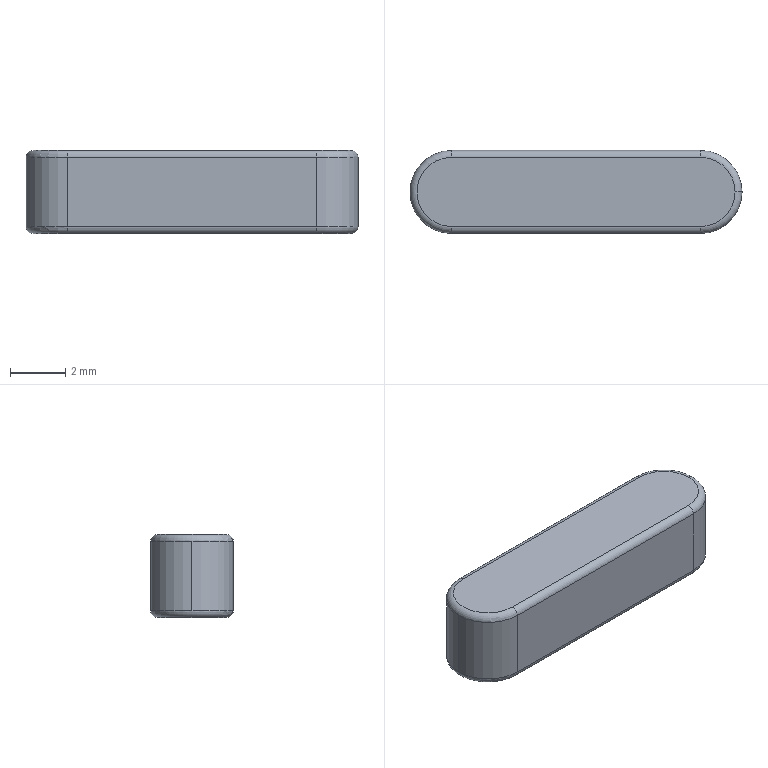Part | STEP file | Type A plain parallel key GB/T 1096 - key 3x3x12 | 1 solid | 17 faces | box 12 x 3 x 3 mm | volume 101.479 mm3 | cylinder 7 | torus 6 | plane 4 | commonest cylinder face diameters 0.5 x4 3 x3
STEP:
#1=CARTESIAN_POINT('',(0.,0.,0.));
#2=DIRECTION('',(0.,0.,1.));
#3=DIRECTION('',(1.,0.,0.));
#4=AXIS2_PLACEMENT_3D('',#1,#2,#3);
#5=CARTESIAN_POINT('',(5.75,0.,0.));
#6=VERTEX_POINT('',#5);
#7=CARTESIAN_POINT('',(4.5,-1.25,0.));
#8=VERTEX_POINT('',#7);
#9=CARTESIAN_POINT('',(4.5,0.,0.));
#10=DIRECTION('',(0.,0.,-1.));
#11=DIRECTION('',(1.,0.,0.));
#12=AXIS2_PLACEMENT_3D('',#9,#10,#11);
#13=CIRCLE('',#12,1.25);
#14=CARTESIAN_POINT('',(4.5,0.,0.25));
#15=DIRECTION('',(0.,0.,1.));
#16=DIRECTION('',(1.,0.,0.));
#17=AXIS2_PLACEMENT_3D('',#14,#15,#16);
#18=TOROIDAL_SURFACE('',#17,1.25,0.25);
#19=CARTESIAN_POINT('',(6.283,4.712));
#20=DIRECTION('',(-1.,0.));
#21=VECTOR('',#20,1.);
#22=LINE('',#19,#21);
#23=(GEOMETRIC_REPRESENTATION_CONTEXT(2)PARAMETRIC_REPRESENTATION_CONTEXT()REPRESENTATION_CONTEXT('',''));
#24=DEFINITIONAL_REPRESENTATION('',(#22),#23);
#25=PCURVE('',#18,#24);
#26=CARTESIAN_POINT('',(-4.5,0.,0.));
#27=DIRECTION('',(0.,0.,1.));
#28=DIRECTION('',(1.,0.,0.));
#29=AXIS2_PLACEMENT_3D('',#26,#27,#28);
#30=PLANE('',#29);
#31=CARTESIAN_POINT('',(10.25,0.));
#32=CARTESIAN_POINT('',(10.25,-2.165));
#33=CARTESIAN_POINT('',(8.375,-1.083));
#34=CARTESIAN_POINT('',(6.5,0.));
#35=CARTESIAN_POINT('',(8.375,1.083));
#36=CARTESIAN_POINT('',(10.25,2.165));
#37=CARTESIAN_POINT('',(10.25,0.));
#38=(BOUNDED_CURVE()B_SPLINE_CURVE(2,(#31,#32,#33,#34,#35,#36,#37),.UNSPECIFIED.,.T.,.F.)B_SPLINE_CURVE_WITH_KNOTS((1,2,2,2,2,1),(-2.094,0.,2.094,4.189,6.283,8.378),.UNSPECIFIED.)CURVE()GEOMETRIC_REPRESENTATION_ITEM()RATIONAL_B_SPLINE_CURVE((1.,0.5,1.,0.5,1.,0.5,1.))REPRESENTATION_ITEM(''));
#39=(GEOMETRIC_REPRESENTATION_CONTEXT(2)PARAMETRIC_REPRESENTATION_CONTEXT()REPRESENTATION_CONTEXT('',''));
#40=DEFINITIONAL_REPRESENTATION('',(#38),#39);
#41=PCURVE('',#30,#40);
#42=SURFACE_CURVE('',#13,(#25,#41),.PCURVE_S1.);
#43=EDGE_CURVE('',#6,#8,#42,.T.);
#44=ORIENTED_EDGE('',*,*,#43,.F.);
#45=CARTESIAN_POINT('',(6.,0.,0.25));
#46=VERTEX_POINT('',#45);
#47=CARTESIAN_POINT('',(5.75,0.,0.25));
#48=DIRECTION('',(0.,-1.,0.));
#49=DIRECTION('',(0.,0.,-1.));
#50=AXIS2_PLACEMENT_3D('',#47,#48,#49);
#51=CIRCLE('',#50,0.25);
#52=CARTESIAN_POINT('',(6.283,4.712));
#53=DIRECTION('',(0.,1.));
#54=VECTOR('',#53,1.);
#55=LINE('',#52,#54);
#56=(GEOMETRIC_REPRESENTATION_CONTEXT(2)PARAMETRIC_REPRESENTATION_CONTEXT()REPRESENTATION_CONTEXT('',''));
#57=DEFINITIONAL_REPRESENTATION('',(#55),#56);
#58=PCURVE('',#18,#57);
#59=CARTESIAN_POINT('',(4.5,0.,0.25));
#60=DIRECTION('',(0.,0.,1.));
#61=DIRECTION('',(1.,0.,0.));
#62=AXIS2_PLACEMENT_3D('',#59,#60,#61);
#63=TOROIDAL_SURFACE('',#62,1.25,0.25);
#64=CARTESIAN_POINT('',(0.,4.712));
#65=DIRECTION('',(0.,1.));
#66=VECTOR('',#65,1.);
#67=LINE('',#64,#66);
#68=(GEOMETRIC_REPRESENTATION_CONTEXT(2)PARAMETRIC_REPRESENTATION_CONTEXT()REPRESENTATION_CONTEXT('',''));
#69=DEFINITIONAL_REPRESENTATION('',(#67),#68);
#70=PCURVE('',#63,#69);
#71=SURFACE_CURVE('',#51,(#58,#70),.PCURVE_S1.);
#72=EDGE_CURVE('',#6,#46,#71,.T.);
#73=ORIENTED_EDGE('',*,*,#72,.T.);
#74=CARTESIAN_POINT('',(4.5,-1.5,0.25));
#75=VERTEX_POINT('',#74);
#76=CARTESIAN_POINT('',(4.5,0.,0.25));
#77=DIRECTION('',(0.,0.,1.));
#78=DIRECTION('',(1.,0.,0.));
#79=AXIS2_PLACEMENT_3D('',#76,#77,#78);
#80=CIRCLE('',#79,1.5);
#81=CARTESIAN_POINT('',(0.,6.283));
#82=DIRECTION('',(1.,0.));
#83=VECTOR('',#82,1.);
#84=LINE('',#81,#83);
#85=(GEOMETRIC_REPRESENTATION_CONTEXT(2)PARAMETRIC_REPRESENTATION_CONTEXT()REPRESENTATION_CONTEXT('',''));
#86=DEFINITIONAL_REPRESENTATION('',(#84),#85);
#87=PCURVE('',#18,#86);
#88=CARTESIAN_POINT('',(4.5,0.,3.));
#89=DIRECTION('',(0.,0.,-1.));
#90=DIRECTION('',(-1.,0.,0.));
#91=AXIS2_PLACEMENT_3D('',#88,#89,#90);
#92=CYLINDRICAL_SURFACE('',#91,1.5);
#93=CARTESIAN_POINT('',(9.425,2.75));
#94=DIRECTION('',(-1.,0.));
#95=VECTOR('',#94,1.);
#96=LINE('',#93,#95);
#97=(GEOMETRIC_REPRESENTATION_CONTEXT(2)PARAMETRIC_REPRESENTATION_CONTEXT()REPRESENTATION_CONTEXT('',''));
#98=DEFINITIONAL_REPRESENTATION('',(#96),#97);
#99=PCURVE('',#92,#98);
#100=SURFACE_CURVE('',#80,(#87,#99),.PCURVE_S1.);
#101=EDGE_CURVE('',#75,#46,#100,.T.);
#102=ORIENTED_EDGE('',*,*,#101,.F.);
#103=CARTESIAN_POINT('',(4.5,-1.25,0.25));
#104=DIRECTION('',(1.,0.,0.));
#105=DIRECTION('',(0.,0.,-1.));
#106=AXIS2_PLACEMENT_3D('',#103,#104,#105);
#107=CIRCLE('',#106,0.25);
#108=CARTESIAN_POINT('',(4.712,10.996));
#109=DIRECTION('',(0.,-1.));
#110=VECTOR('',#109,1.);
#111=LINE('',#108,#110);
#112=(GEOMETRIC_REPRESENTATION_CONTEXT(2)PARAMETRIC_REPRESENTATION_CONTEXT()REPRESENTATION_CONTEXT('',''));
#113=DEFINITIONAL_REPRESENTATION('',(#111),#112);
#114=PCURVE('',#18,#113);
#115=CARTESIAN_POINT('',(-4.5,-1.25,0.25));
#116=DIRECTION('',(1.,0.,0.));
#117=DIRECTION('',(0.,1.,0.));
#118=AXIS2_PLACEMENT_3D('',#115,#116,#117);
#119=CYLINDRICAL_SURFACE('',#118,0.25);
#120=CARTESIAN_POINT('',(-1.571,9.));
#121=DIRECTION('',(1.,0.));
#122=VECTOR('',#121,1.);
#123=LINE('',#120,#122);
#124=(GEOMETRIC_REPRESENTATION_CONTEXT(2)PARAMETRIC_REPRESENTATION_CONTEXT()REPRESENTATION_CONTEXT('',''));
#125=DEFINITIONAL_REPRESENTATION('',(#123),#124);
#126=PCURVE('',#119,#125);
#127=SURFACE_CURVE('',#107,(#114,#126),.PCURVE_S1.);
#128=EDGE_CURVE('',#75,#8,#127,.T.);
#129=ORIENTED_EDGE('',*,*,#128,.T.);
#130=EDGE_LOOP('',(#44,#73,#102,#129));
#131=FACE_BOUND('',#130,.T.);
#132=ADVANCED_FACE('',(#131),#18,.T.);
#133=CARTESIAN_POINT('',(6.,0.,2.75));
#134=VERTEX_POINT('',#133);
#135=CARTESIAN_POINT('',(4.5,-1.5,2.75));
#136=VERTEX_POINT('',#135);
#137=CARTESIAN_POINT('',(4.5,0.,2.75));
#138=DIRECTION('',(0.,0.,-1.));
#139=DIRECTION('',(1.,0.,0.));
#140=AXIS2_PLACEMENT_3D('',#137,#138,#139);
#141=CIRCLE('',#140,1.5);
#142=CARTESIAN_POINT('',(4.5,0.,2.75));
#143=DIRECTION('',(0.,0.,1.));
#144=DIRECTION('',(1.,0.,0.));
#145=AXIS2_PLACEMENT_3D('',#142,#143,#144);
#146=TOROIDAL_SURFACE('',#145,1.25,0.25);
#147=CARTESIAN_POINT('',(6.283,0.));
#148=DIRECTION('',(-1.,0.));
#149=VECTOR('',#148,1.);
#150=LINE('',#147,#149);
#151=(GEOMETRIC_REPRESENTATION_CONTEXT(2)PARAMETRIC_REPRESENTATION_CONTEXT()REPRESENTATION_CONTEXT('',''));
#152=DEFINITIONAL_REPRESENTATION('',(#150),#151);
#153=PCURVE('',#146,#152);
#154=CARTESIAN_POINT('',(3.142,0.25));
#155=DIRECTION('',(1.,0.));
#156=VECTOR('',#155,1.);
#157=LINE('',#154,#156);
#158=(GEOMETRIC_REPRESENTATION_CONTEXT(2)PARAMETRIC_REPRESENTATION_CONTEXT()REPRESENTATION_CONTEXT('',''));
#159=DEFINITIONAL_REPRESENTATION('',(#157),#158);
#160=PCURVE('',#92,#159);
#161=SURFACE_CURVE('',#141,(#153,#160),.PCURVE_S1.);
#162=EDGE_CURVE('',#134,#136,#161,.T.);
#163=ORIENTED_EDGE('',*,*,#162,.F.);
#164=CARTESIAN_POINT('',(5.75,0.,3.));
#165=VERTEX_POINT('',#164);
#166=CARTESIAN_POINT('',(5.75,0.,2.75));
#167=DIRECTION('',(0.,-1.,0.));
#168=DIRECTION('',(0.,0.,-1.));
#169=AXIS2_PLACEMENT_3D('',#166,#167,#168);
#170=CIRCLE('',#169,0.25);
#171=CARTESIAN_POINT('',(6.283,-1.571));
#172=DIRECTION('',(0.,1.));
#173=VECTOR('',#172,1.);
#174=LINE('',#171,#173);
#175=(GEOMETRIC_REPRESENTATION_CONTEXT(2)PARAMETRIC_REPRESENTATION_CONTEXT()REPRESENTATION_CONTEXT('',''));
#176=DEFINITIONAL_REPRESENTATION('',(#174),#175);
#177=PCURVE('',#146,#176);
#178=CARTESIAN_POINT('',(4.5,0.,2.75));
#179=DIRECTION('',(0.,0.,1.));
#180=DIRECTION('',(1.,0.,0.));
#181=AXIS2_PLACEMENT_3D('',#178,#179,#180);
#182=TOROIDAL_SURFACE('',#181,1.25,0.25);
#183=CARTESIAN_POINT('',(0.,-1.571));
#184=DIRECTION('',(0.,1.));
#185=VECTOR('',#184,1.);
#186=LINE('',#183,#185);
#187=(GEOMETRIC_REPRESENTATION_CONTEXT(2)PARAMETRIC_REPRESENTATION_CONTEXT()REPRESENTATION_CONTEXT('',''));
#188=DEFINITIONAL_REPRESENTATION('',(#186),#187);
#189=PCURVE('',#182,#188);
#190=SURFACE_CURVE('',#170,(#177,#189),.PCURVE_S1.);
#191=EDGE_CURVE('',#134,#165,#190,.T.);
#192=ORIENTED_EDGE('',*,*,#191,.T.);
#193=CARTESIAN_POINT('',(4.5,-1.25,3.));
#194=VERTEX_POINT('',#193);
#195=CARTESIAN_POINT('',(4.5,0.,3.));
#196=DIRECTION('',(0.,0.,1.));
#197=DIRECTION('',(1.,0.,0.));
#198=AXIS2_PLACEMENT_3D('',#195,#196,#197);
#199=CIRCLE('',#198,1.25);
#200=CARTESIAN_POINT('',(0.,1.571));
#201=DIRECTION('',(1.,0.));
#202=VECTOR('',#201,1.);
#203=LINE('',#200,#202);
#204=(GEOMETRIC_REPRESENTATION_CONTEXT(2)PARAMETRIC_REPRESENTATION_CONTEXT()REPRESENTATION_CONTEXT('',''));
#205=DEFINITIONAL_REPRESENTATION('',(#203),#204);
#206=PCURVE('',#146,#205);
#207=CARTESIAN_POINT('',(-4.5,0.,3.));
#208=DIRECTION('',(0.,0.,1.));
#209=DIRECTION('',(1.,0.,0.));
#210=AXIS2_PLACEMENT_3D('',#207,#208,#209);
#211=PLANE('',#210);
#212=CARTESIAN_POINT('',(9.,0.));
#213=DIRECTION('',(1.,0.));
#214=AXIS2_PLACEMENT_2D('',#212,#213);
#215=CIRCLE('',#214,1.25);
#216=(GEOMETRIC_REPRESENTATION_CONTEXT(2)PARAMETRIC_REPRESENTATION_CONTEXT()REPRESENTATION_CONTEXT('',''));
#217=DEFINITIONAL_REPRESENTATION('',(#215),#216);
#218=PCURVE('',#211,#217);
#219=SURFACE_CURVE('',#199,(#206,#218),.PCURVE_S1.);
#220=EDGE_CURVE('',#194,#165,#219,.T.);
#221=ORIENTED_EDGE('',*,*,#220,.F.);
#222=CARTESIAN_POINT('',(4.5,-1.25,2.75));
#223=DIRECTION('',(1.,0.,0.));
#224=DIRECTION('',(0.,0.,-1.));
#225=AXIS2_PLACEMENT_3D('',#222,#223,#224);
#226=CIRCLE('',#225,0.25);
#227=CARTESIAN_POINT('',(4.712,4.712));
#228=DIRECTION('',(0.,-1.));
#229=VECTOR('',#228,1.);
#230=LINE('',#227,#229);
#231=(GEOMETRIC_REPRESENTATION_CONTEXT(2)PARAMETRIC_REPRESENTATION_CONTEXT()REPRESENTATION_CONTEXT('',''));
#232=DEFINITIONAL_REPRESENTATION('',(#230),#231);
#233=PCURVE('',#146,#232);
#234=CARTESIAN_POINT('',(-4.5,-1.25,2.75));
#235=DIRECTION('',(-1.,0.,0.));
#236=DIRECTION('',(0.,-1.,0.));
#237=AXIS2_PLACEMENT_3D('',#234,#235,#236);
#238=CYLINDRICAL_SURFACE('',#237,0.25);
#239=CARTESIAN_POINT('',(4.712,-9.));
#240=DIRECTION('',(-1.,0.));
#241=VECTOR('',#240,1.);
#242=LINE('',#239,#241);
#243=(GEOMETRIC_REPRESENTATION_CONTEXT(2)PARAMETRIC_REPRESENTATION_CONTEXT()REPRESENTATION_CONTEXT('',''));
#244=DEFINITIONAL_REPRESENTATION('',(#242),#243);
#245=PCURVE('',#238,#244);
#246=SURFACE_CURVE('',#226,(#233,#245),.PCURVE_S1.);
#247=EDGE_CURVE('',#194,#136,#246,.T.);
#248=ORIENTED_EDGE('',*,*,#247,.T.);
#249=EDGE_LOOP('',(#163,#192,#221,#248));
#250=FACE_BOUND('',#249,.T.);
#251=ADVANCED_FACE('',(#250),#146,.T.);
#252=CARTESIAN_POINT('',(-4.5,-1.5,2.75));
#253=VERTEX_POINT('',#252);
#254=CARTESIAN_POINT('',(-6.,0.,2.75));
#255=VERTEX_POINT('',#254);
#256=CARTESIAN_POINT('',(-4.5,0.,2.75));
#257=DIRECTION('',(0.,0.,-1.));
#258=DIRECTION('',(1.,0.,0.));
#259=AXIS2_PLACEMENT_3D('',#256,#257,#258);
#260=CIRCLE('',#259,1.5);
#261=CARTESIAN_POINT('',(-4.5,0.,3.));
#262=DIRECTION('',(0.,0.,-1.));
#263=DIRECTION('',(-1.,0.,0.));
#264=AXIS2_PLACEMENT_3D('',#261,#262,#263);
#265=CYLINDRICAL_SURFACE('',#264,1.5);
#266=CARTESIAN_POINT('',(3.142,0.25));
#267=DIRECTION('',(1.,0.));
#268=VECTOR('',#267,1.);
#269=LINE('',#266,#268);
#270=(GEOMETRIC_REPRESENTATION_CONTEXT(2)PARAMETRIC_REPRESENTATION_CONTEXT()REPRESENTATION_CONTEXT('',''));
#271=DEFINITIONAL_REPRESENTATION('',(#269),#270);
#272=PCURVE('',#265,#271);
#273=CARTESIAN_POINT('',(-4.5,0.,2.75));
#274=DIRECTION('',(0.,0.,1.));
#275=DIRECTION('',(1.,0.,0.));
#276=AXIS2_PLACEMENT_3D('',#273,#274,#275);
#277=TOROIDAL_SURFACE('',#276,1.25,0.25);
#278=CARTESIAN_POINT('',(6.283,0.));
#279=DIRECTION('',(-1.,0.));
#280=VECTOR('',#279,1.);
#281=LINE('',#278,#280);
#282=(GEOMETRIC_REPRESENTATION_CONTEXT(2)PARAMETRIC_REPRESENTATION_CONTEXT()REPRESENTATION_CONTEXT('',''));
#283=DEFINITIONAL_REPRESENTATION('',(#281),#282);
#284=PCURVE('',#277,#283);
#285=SURFACE_CURVE('',#260,(#272,#284),.PCURVE_S1.);
#286=EDGE_CURVE('',#253,#255,#285,.T.);
#287=ORIENTED_EDGE('',*,*,#286,.T.);
#288=CARTESIAN_POINT('',(-6.,0.,0.25));
#289=VERTEX_POINT('',#288);
#290=CARTESIAN_POINT('',(-6.,0.,3.));
#291=DIRECTION('',(0.,0.,-1.));
#292=VECTOR('',#291,1.);
#293=LINE('',#290,#292);
#294=CARTESIAN_POINT('',(6.283,0.));
#295=DIRECTION('',(0.,1.));
#296=VECTOR('',#295,1.);
#297=LINE('',#294,#296);
#298=(GEOMETRIC_REPRESENTATION_CONTEXT(2)PARAMETRIC_REPRESENTATION_CONTEXT()REPRESENTATION_CONTEXT('',''));
#299=DEFINITIONAL_REPRESENTATION('',(#297),#298);
#300=PCURVE('',#265,#299);
#301=CARTESIAN_POINT('',(-4.5,0.,3.));
#302=DIRECTION('',(0.,0.,-1.));
#303=DIRECTION('',(-1.,0.,0.));
#304=AXIS2_PLACEMENT_3D('',#301,#302,#303);
#305=CYLINDRICAL_SURFACE('',#304,1.5);
#306=CARTESIAN_POINT('',(0.,0.));
#307=DIRECTION('',(0.,1.));
#308=VECTOR('',#307,1.);
#309=LINE('',#306,#308);
#310=(GEOMETRIC_REPRESENTATION_CONTEXT(2)PARAMETRIC_REPRESENTATION_CONTEXT()REPRESENTATION_CONTEXT('',''));
#311=DEFINITIONAL_REPRESENTATION('',(#309),#310);
#312=PCURVE('',#305,#311);
#313=SURFACE_CURVE('',#293,(#300,#312),.PCURVE_S1.);
#314=EDGE_CURVE('',#255,#289,#313,.T.);
#315=ORIENTED_EDGE('',*,*,#314,.T.);
#316=CARTESIAN_POINT('',(-4.5,-1.5,0.25));
#317=VERTEX_POINT('',#316);
#318=CARTESIAN_POINT('',(-4.5,0.,0.25));
#319=DIRECTION('',(0.,0.,1.));
#320=DIRECTION('',(1.,0.,0.));
#321=AXIS2_PLACEMENT_3D('',#318,#319,#320);
#322=CIRCLE('',#321,1.5);
#323=CARTESIAN_POINT('',(9.425,2.75));
#324=DIRECTION('',(-1.,0.));
#325=VECTOR('',#324,1.);
#326=LINE('',#323,#325);
#327=(GEOMETRIC_REPRESENTATION_CONTEXT(2)PARAMETRIC_REPRESENTATION_CONTEXT()REPRESENTATION_CONTEXT('',''));
#328=DEFINITIONAL_REPRESENTATION('',(#326),#327);
#329=PCURVE('',#265,#328);
#330=CARTESIAN_POINT('',(-4.5,0.,0.25));
#331=DIRECTION('',(0.,0.,1.));
#332=DIRECTION('',(1.,0.,0.));
#333=AXIS2_PLACEMENT_3D('',#330,#331,#332);
#334=TOROIDAL_SURFACE('',#333,1.25,0.25);
#335=CARTESIAN_POINT('',(0.,6.283));
#336=DIRECTION('',(1.,0.));
#337=VECTOR('',#336,1.);
#338=LINE('',#335,#337);
#339=(GEOMETRIC_REPRESENTATION_CONTEXT(2)PARAMETRIC_REPRESENTATION_CONTEXT()REPRESENTATION_CONTEXT('',''));
#340=DEFINITIONAL_REPRESENTATION('',(#338),#339);
#341=PCURVE('',#334,#340);
#342=SURFACE_CURVE('',#322,(#329,#341),.PCURVE_S1.);
#343=EDGE_CURVE('',#289,#317,#342,.T.);
#344=ORIENTED_EDGE('',*,*,#343,.T.);
#345=CARTESIAN_POINT('',(-4.5,-1.5,3.));
#346=DIRECTION('',(0.,0.,-1.));
#347=VECTOR('',#346,1.);
#348=LINE('',#345,#347);
#349=CARTESIAN_POINT('',(4.712,0.));
#350=DIRECTION('',(0.,1.));
#351=VECTOR('',#350,1.);
#352=LINE('',#349,#351);
#353=(GEOMETRIC_REPRESENTATION_CONTEXT(2)PARAMETRIC_REPRESENTATION_CONTEXT()REPRESENTATION_CONTEXT('',''));
#354=DEFINITIONAL_REPRESENTATION('',(#352),#353);
#355=PCURVE('',#265,#354);
#356=CARTESIAN_POINT('',(-4.5,-1.5,3.));
#357=DIRECTION('',(0.,1.,0.));
#358=DIRECTION('',(-1.,0.,0.));
#359=AXIS2_PLACEMENT_3D('',#356,#357,#358);
#360=PLANE('',#359);
#361=CARTESIAN_POINT('',(0.,0.));
#362=DIRECTION('',(0.,-1.));
#363=VECTOR('',#362,1.);
#364=LINE('',#361,#363);
#365=(GEOMETRIC_REPRESENTATION_CONTEXT(2)PARAMETRIC_REPRESENTATION_CONTEXT()REPRESENTATION_CONTEXT('',''));
#366=DEFINITIONAL_REPRESENTATION('',(#364),#365);
#367=PCURVE('',#360,#366);
#368=SURFACE_CURVE('',#348,(#355,#367),.PCURVE_S1.);
#369=EDGE_CURVE('',#253,#317,#368,.T.);
#370=ORIENTED_EDGE('',*,*,#369,.F.);
#371=EDGE_LOOP('',(#287,#315,#344,#370));
#372=FACE_BOUND('',#371,.T.);
#373=ADVANCED_FACE('',(#372),#265,.T.);
#374=ORIENTED_EDGE('',*,*,#314,.F.);
#375=CARTESIAN_POINT('',(-4.5,1.5,2.75));
#376=VERTEX_POINT('',#375);
#377=CARTESIAN_POINT('',(-4.5,0.,2.75));
#378=DIRECTION('',(0.,0.,-1.));
#379=DIRECTION('',(1.,0.,0.));
#380=AXIS2_PLACEMENT_3D('',#377,#378,#379);
#381=CIRCLE('',#380,1.5);
#382=CARTESIAN_POINT('',(-3.142,0.25));
#383=DIRECTION('',(1.,0.));
#384=VECTOR('',#383,1.);
#385=LINE('',#382,#384);
#386=(GEOMETRIC_REPRESENTATION_CONTEXT(2)PARAMETRIC_REPRESENTATION_CONTEXT()REPRESENTATION_CONTEXT('',''));
#387=DEFINITIONAL_REPRESENTATION('',(#385),#386);
#388=PCURVE('',#305,#387);
#389=CARTESIAN_POINT('',(6.283,0.));
#390=DIRECTION('',(-1.,0.));
#391=VECTOR('',#390,1.);
#392=LINE('',#389,#391);
#393=(GEOMETRIC_REPRESENTATION_CONTEXT(2)PARAMETRIC_REPRESENTATION_CONTEXT()REPRESENTATION_CONTEXT('',''));
#394=DEFINITIONAL_REPRESENTATION('',(#392),#393);
#395=PCURVE('',#277,#394);
#396=SURFACE_CURVE('',#381,(#388,#395),.PCURVE_S1.);
#397=EDGE_CURVE('',#255,#376,#396,.T.);
#398=ORIENTED_EDGE('',*,*,#397,.T.);
#399=CARTESIAN_POINT('',(-4.5,1.5,0.25));
#400=VERTEX_POINT('',#399);
#401=CARTESIAN_POINT('',(-4.5,1.5,3.));
#402=DIRECTION('',(0.,0.,-1.));
#403=VECTOR('',#402,1.);
#404=LINE('',#401,#403);
#405=CARTESIAN_POINT('',(1.571,0.));
#406=DIRECTION('',(0.,1.));
#407=VECTOR('',#406,1.);
#408=LINE('',#405,#407);
#409=(GEOMETRIC_REPRESENTATION_CONTEXT(2)PARAMETRIC_REPRESENTATION_CONTEXT()REPRESENTATION_CONTEXT('',''));
#410=DEFINITIONAL_REPRESENTATION('',(#408),#409);
#411=PCURVE('',#305,#410);
#412=CARTESIAN_POINT('',(-4.5,1.5,3.));
#413=DIRECTION('',(0.,-1.,0.));
#414=DIRECTION('',(1.,0.,0.));
#415=AXIS2_PLACEMENT_3D('',#412,#413,#414);
#416=PLANE('',#415);
#417=CARTESIAN_POINT('',(0.,0.));
#418=DIRECTION('',(0.,-1.));
#419=VECTOR('',#418,1.);
#420=LINE('',#417,#419);
#421=(GEOMETRIC_REPRESENTATION_CONTEXT(2)PARAMETRIC_REPRESENTATION_CONTEXT()REPRESENTATION_CONTEXT('',''));
#422=DEFINITIONAL_REPRESENTATION('',(#420),#421);
#423=PCURVE('',#416,#422);
#424=SURFACE_CURVE('',#404,(#411,#423),.PCURVE_S1.);
#425=EDGE_CURVE('',#376,#400,#424,.T.);
#426=ORIENTED_EDGE('',*,*,#425,.T.);
#427=CARTESIAN_POINT('',(-4.5,0.,0.25));
#428=DIRECTION('',(0.,0.,1.));
#429=DIRECTION('',(1.,0.,0.));
#430=AXIS2_PLACEMENT_3D('',#427,#428,#429);
#431=CIRCLE('',#430,1.5);
#432=CARTESIAN_POINT('',(3.142,2.75));
#433=DIRECTION('',(-1.,0.));
#434=VECTOR('',#433,1.);
#435=LINE('',#432,#434);
#436=(GEOMETRIC_REPRESENTATION_CONTEXT(2)PARAMETRIC_REPRESENTATION_CONTEXT()REPRESENTATION_CONTEXT('',''));
#437=DEFINITIONAL_REPRESENTATION('',(#435),#436);
#438=PCURVE('',#305,#437);
#439=CARTESIAN_POINT('',(0.,6.283));
#440=DIRECTION('',(1.,0.));
#441=VECTOR('',#440,1.);
#442=LINE('',#439,#441);
#443=(GEOMETRIC_REPRESENTATION_CONTEXT(2)PARAMETRIC_REPRESENTATION_CONTEXT()REPRESENTATION_CONTEXT('',''));
#444=DEFINITIONAL_REPRESENTATION('',(#442),#443);
#445=PCURVE('',#334,#444);
#446=SURFACE_CURVE('',#431,(#438,#445),.PCURVE_S1.);
#447=EDGE_CURVE('',#400,#289,#446,.T.);
#448=ORIENTED_EDGE('',*,*,#447,.T.);
#449=EDGE_LOOP('',(#374,#398,#426,#448));
#450=FACE_BOUND('',#449,.T.);
#451=ADVANCED_FACE('',(#450),#305,.T.);
#452=CARTESIAN_POINT('',(4.5,-1.5,3.));
#453=DIRECTION('',(0.,0.,-1.));
#454=VECTOR('',#453,1.);
#455=LINE('',#452,#454);
#456=CARTESIAN_POINT('',(-9.,0.));
#457=DIRECTION('',(0.,-1.));
#458=VECTOR('',#457,1.);
#459=LINE('',#456,#458);
#460=(GEOMETRIC_REPRESENTATION_CONTEXT(2)PARAMETRIC_REPRESENTATION_CONTEXT()REPRESENTATION_CONTEXT('',''));
#461=DEFINITIONAL_REPRESENTATION('',(#459),#460);
#462=PCURVE('',#360,#461);
#463=CARTESIAN_POINT('',(4.712,0.));
#464=DIRECTION('',(0.,1.));
#465=VECTOR('',#464,1.);
#466=LINE('',#463,#465);
#467=(GEOMETRIC_REPRESENTATION_CONTEXT(2)PARAMETRIC_REPRESENTATION_CONTEXT()REPRESENTATION_CONTEXT('',''));
#468=DEFINITIONAL_REPRESENTATION('',(#466),#467);
#469=PCURVE('',#92,#468);
#470=SURFACE_CURVE('',#455,(#462,#469),.PCURVE_S1.);
#471=EDGE_CURVE('',#136,#75,#470,.T.);
#472=ORIENTED_EDGE('',*,*,#471,.F.);
#473=CARTESIAN_POINT('',(-4.5,-1.5,2.75));
#474=DIRECTION('',(-1.,0.,0.));
#475=VECTOR('',#474,1.);
#476=LINE('',#473,#475);
#477=CARTESIAN_POINT('',(0.,-0.25));
#478=DIRECTION('',(1.,0.));
#479=VECTOR('',#478,1.);
#480=LINE('',#477,#479);
#481=(GEOMETRIC_REPRESENTATION_CONTEXT(2)PARAMETRIC_REPRESENTATION_CONTEXT()REPRESENTATION_CONTEXT('',''));
#482=DEFINITIONAL_REPRESENTATION('',(#480),#481);
#483=PCURVE('',#360,#482);
#484=CARTESIAN_POINT('',(0.,0.));
#485=DIRECTION('',(0.,1.));
#486=VECTOR('',#485,1.);
#487=LINE('',#484,#486);
#488=(GEOMETRIC_REPRESENTATION_CONTEXT(2)PARAMETRIC_REPRESENTATION_CONTEXT()REPRESENTATION_CONTEXT('',''));
#489=DEFINITIONAL_REPRESENTATION('',(#487),#488);
#490=PCURVE('',#238,#489);
#491=SURFACE_CURVE('',#476,(#483,#490),.PCURVE_S1.);
#492=EDGE_CURVE('',#136,#253,#491,.T.);
#493=ORIENTED_EDGE('',*,*,#492,.T.);
#494=ORIENTED_EDGE('',*,*,#369,.T.);
#495=CARTESIAN_POINT('',(-4.5,-1.5,0.25));
#496=DIRECTION('',(1.,0.,0.));
#497=VECTOR('',#496,1.);
#498=LINE('',#495,#497);
#499=CARTESIAN_POINT('',(0.,-2.75));
#500=DIRECTION('',(-1.,0.));
#501=VECTOR('',#500,1.);
#502=LINE('',#499,#501);
#503=(GEOMETRIC_REPRESENTATION_CONTEXT(2)PARAMETRIC_REPRESENTATION_CONTEXT()REPRESENTATION_CONTEXT('',''));
#504=DEFINITIONAL_REPRESENTATION('',(#502),#503);
#505=PCURVE('',#360,#504);
#506=CARTESIAN_POINT('',(3.142,0.));
#507=DIRECTION('',(0.,1.));
#508=VECTOR('',#507,1.);
#509=LINE('',#506,#508);
#510=(GEOMETRIC_REPRESENTATION_CONTEXT(2)PARAMETRIC_REPRESENTATION_CONTEXT()REPRESENTATION_CONTEXT('',''));
#511=DEFINITIONAL_REPRESENTATION('',(#509),#510);
#512=PCURVE('',#119,#511);
#513=SURFACE_CURVE('',#498,(#505,#512),.PCURVE_S1.);
#514=EDGE_CURVE('',#317,#75,#513,.T.);
#515=ORIENTED_EDGE('',*,*,#514,.T.);
#516=EDGE_LOOP('',(#472,#493,#494,#515));
#517=FACE_BOUND('',#516,.T.);
#518=ADVANCED_FACE('',(#517),#360,.F.);
#519=CARTESIAN_POINT('',(4.5,1.5,2.75));
#520=VERTEX_POINT('',#519);
#521=CARTESIAN_POINT('',(4.5,1.5,0.25));
#522=VERTEX_POINT('',#521);
#523=CARTESIAN_POINT('',(4.5,1.5,3.));
#524=DIRECTION('',(0.,0.,-1.));
#525=VECTOR('',#524,1.);
#526=LINE('',#523,#525);
#527=CARTESIAN_POINT('',(1.571,0.));
#528=DIRECTION('',(0.,1.));
#529=VECTOR('',#528,1.);
#530=LINE('',#527,#529);
#531=(GEOMETRIC_REPRESENTATION_CONTEXT(2)PARAMETRIC_REPRESENTATION_CONTEXT()REPRESENTATION_CONTEXT('',''));
#532=DEFINITIONAL_REPRESENTATION('',(#530),#531);
#533=PCURVE('',#92,#532);
#534=CARTESIAN_POINT('',(9.,0.));
#535=DIRECTION('',(0.,-1.));
#536=VECTOR('',#535,1.);
#537=LINE('',#534,#536);
#538=(GEOMETRIC_REPRESENTATION_CONTEXT(2)PARAMETRIC_REPRESENTATION_CONTEXT()REPRESENTATION_CONTEXT('',''));
#539=DEFINITIONAL_REPRESENTATION('',(#537),#538);
#540=PCURVE('',#416,#539);
#541=SURFACE_CURVE('',#526,(#533,#540),.PCURVE_S1.);
#542=EDGE_CURVE('',#520,#522,#541,.T.);
#543=ORIENTED_EDGE('',*,*,#542,.F.);
#544=CARTESIAN_POINT('',(4.5,0.,2.75));
#545=DIRECTION('',(0.,0.,-1.));
#546=DIRECTION('',(1.,0.,0.));
#547=AXIS2_PLACEMENT_3D('',#544,#545,#546);
#548=CIRCLE('',#547,1.5);
#549=CARTESIAN_POINT('',(-3.142,0.25));
#550=DIRECTION('',(1.,0.));
#551=VECTOR('',#550,1.);
#552=LINE('',#549,#551);
#553=(GEOMETRIC_REPRESENTATION_CONTEXT(2)PARAMETRIC_REPRESENTATION_CONTEXT()REPRESENTATION_CONTEXT('',''));
#554=DEFINITIONAL_REPRESENTATION('',(#552),#553);
#555=PCURVE('',#92,#554);
#556=CARTESIAN_POINT('',(6.283,0.));
#557=DIRECTION('',(-1.,0.));
#558=VECTOR('',#557,1.);
#559=LINE('',#556,#558);
#560=(GEOMETRIC_REPRESENTATION_CONTEXT(2)PARAMETRIC_REPRESENTATION_CONTEXT()REPRESENTATION_CONTEXT('',''));
#561=DEFINITIONAL_REPRESENTATION('',(#559),#560);
#562=PCURVE('',#182,#561);
#563=SURFACE_CURVE('',#548,(#555,#562),.PCURVE_S1.);
#564=EDGE_CURVE('',#520,#134,#563,.T.);
#565=ORIENTED_EDGE('',*,*,#564,.T.);
#566=ORIENTED_EDGE('',*,*,#162,.T.);
#567=ORIENTED_EDGE('',*,*,#471,.T.);
#568=ORIENTED_EDGE('',*,*,#101,.T.);
#569=CARTESIAN_POINT('',(4.5,0.,0.25));
#570=DIRECTION('',(0.,0.,1.));
#571=DIRECTION('',(1.,0.,0.));
#572=AXIS2_PLACEMENT_3D('',#569,#570,#571);
#573=CIRCLE('',#572,1.5);
#574=CARTESIAN_POINT('',(3.142,2.75));
#575=DIRECTION('',(-1.,0.));
#576=VECTOR('',#575,1.);
#577=LINE('',#574,#576);
#578=(GEOMETRIC_REPRESENTATION_CONTEXT(2)PARAMETRIC_REPRESENTATION_CONTEXT()REPRESENTATION_CONTEXT('',''));
#579=DEFINITIONAL_REPRESENTATION('',(#577),#578);
#580=PCURVE('',#92,#579);
#581=CARTESIAN_POINT('',(0.,6.283));
#582=DIRECTION('',(1.,0.));
#583=VECTOR('',#582,1.);
#584=LINE('',#581,#583);
#585=(GEOMETRIC_REPRESENTATION_CONTEXT(2)PARAMETRIC_REPRESENTATION_CONTEXT()REPRESENTATION_CONTEXT('',''));
#586=DEFINITIONAL_REPRESENTATION('',(#584),#585);
#587=PCURVE('',#63,#586);
#588=SURFACE_CURVE('',#573,(#580,#587),.PCURVE_S1.);
#589=EDGE_CURVE('',#46,#522,#588,.T.);
#590=ORIENTED_EDGE('',*,*,#589,.T.);
#591=EDGE_LOOP('',(#543,#565,#566,#567,#568,#590));
#592=FACE_BOUND('',#591,.T.);
#593=ADVANCED_FACE('',(#592),#92,.T.);
#594=ORIENTED_EDGE('',*,*,#425,.F.);
#595=CARTESIAN_POINT('',(4.5,1.5,2.75));
#596=DIRECTION('',(1.,0.,0.));
#597=VECTOR('',#596,1.);
#598=LINE('',#595,#597);
#599=CARTESIAN_POINT('',(9.,-0.25));
#600=DIRECTION('',(1.,0.));
#601=VECTOR('',#600,1.);
#602=LINE('',#599,#601);
#603=(GEOMETRIC_REPRESENTATION_CONTEXT(2)PARAMETRIC_REPRESENTATION_CONTEXT()REPRESENTATION_CONTEXT('',''));
#604=DEFINITIONAL_REPRESENTATION('',(#602),#603);
#605=PCURVE('',#416,#604);
#606=CARTESIAN_POINT('',(-4.5,1.25,2.75));
#607=DIRECTION('',(1.,0.,0.));
#608=DIRECTION('',(0.,1.,0.));
#609=AXIS2_PLACEMENT_3D('',#606,#607,#608);
#610=CYLINDRICAL_SURFACE('',#609,0.25);
#611=CARTESIAN_POINT('',(0.,9.));
#612=DIRECTION('',(0.,1.));
#613=VECTOR('',#612,1.);
#614=LINE('',#611,#613);
#615=(GEOMETRIC_REPRESENTATION_CONTEXT(2)PARAMETRIC_REPRESENTATION_CONTEXT()REPRESENTATION_CONTEXT('',''));
#616=DEFINITIONAL_REPRESENTATION('',(#614),#615);
#617=PCURVE('',#610,#616);
#618=SURFACE_CURVE('',#598,(#605,#617),.PCURVE_S1.);
#619=EDGE_CURVE('',#376,#520,#618,.T.);
#620=ORIENTED_EDGE('',*,*,#619,.T.);
#621=ORIENTED_EDGE('',*,*,#542,.T.);
#622=CARTESIAN_POINT('',(-4.5,1.5,0.25));
#623=DIRECTION('',(-1.,0.,0.));
#624=VECTOR('',#623,1.);
#625=LINE('',#622,#624);
#626=CARTESIAN_POINT('',(0.,-2.75));
#627=DIRECTION('',(-1.,0.));
#628=VECTOR('',#627,1.);
#629=LINE('',#626,#628);
#630=(GEOMETRIC_REPRESENTATION_CONTEXT(2)PARAMETRIC_REPRESENTATION_CONTEXT()REPRESENTATION_CONTEXT('',''));
#631=DEFINITIONAL_REPRESENTATION('',(#629),#630);
#632=PCURVE('',#416,#631);
#633=CARTESIAN_POINT('',(-4.5,1.25,0.25));
#634=DIRECTION('',(-1.,0.,0.));
#635=DIRECTION('',(0.,-1.,0.));
#636=AXIS2_PLACEMENT_3D('',#633,#634,#635);
#637=CYLINDRICAL_SURFACE('',#636,0.25);
#638=CARTESIAN_POINT('',(3.142,0.));
#639=DIRECTION('',(0.,1.));
#640=VECTOR('',#639,1.);
#641=LINE('',#638,#640);
#642=(GEOMETRIC_REPRESENTATION_CONTEXT(2)PARAMETRIC_REPRESENTATION_CONTEXT()REPRESENTATION_CONTEXT('',''));
#643=DEFINITIONAL_REPRESENTATION('',(#641),#642);
#644=PCURVE('',#637,#643);
#645=SURFACE_CURVE('',#625,(#632,#644),.PCURVE_S1.);
#646=EDGE_CURVE('',#522,#400,#645,.T.);
#647=ORIENTED_EDGE('',*,*,#646,.T.);
#648=EDGE_LOOP('',(#594,#620,#621,#647));
#649=FACE_BOUND('',#648,.T.);
#650=ADVANCED_FACE('',(#649),#416,.F.);
#651=CARTESIAN_POINT('',(-4.5,-1.25,3.));
#652=VERTEX_POINT('',#651);
#653=CARTESIAN_POINT('',(4.5,-1.25,3.));
#654=DIRECTION('',(1.,0.,0.));
#655=VECTOR('',#654,1.);
#656=LINE('',#653,#655);
#657=CARTESIAN_POINT('',(9.,-1.25));
#658=DIRECTION('',(1.,0.));
#659=VECTOR('',#658,1.);
#660=LINE('',#657,#659);
#661=(GEOMETRIC_REPRESENTATION_CONTEXT(2)PARAMETRIC_REPRESENTATION_CONTEXT()REPRESENTATION_CONTEXT('',''));
#662=DEFINITIONAL_REPRESENTATION('',(#660),#661);
#663=PCURVE('',#211,#662);
#664=CARTESIAN_POINT('',(1.571,-9.));
#665=DIRECTION('',(0.,-1.));
#666=VECTOR('',#665,1.);
#667=LINE('',#664,#666);
#668=(GEOMETRIC_REPRESENTATION_CONTEXT(2)PARAMETRIC_REPRESENTATION_CONTEXT()REPRESENTATION_CONTEXT('',''));
#669=DEFINITIONAL_REPRESENTATION('',(#667),#668);
#670=PCURVE('',#238,#669);
#671=SURFACE_CURVE('',#656,(#663,#670),.PCURVE_S1.);
#672=EDGE_CURVE('',#652,#194,#671,.T.);
#673=ORIENTED_EDGE('',*,*,#672,.T.);
#674=ORIENTED_EDGE('',*,*,#220,.T.);
#675=CARTESIAN_POINT('',(4.5,1.25,3.));
#676=VERTEX_POINT('',#675);
#677=CARTESIAN_POINT('',(4.5,0.,3.));
#678=DIRECTION('',(0.,0.,1.));
#679=DIRECTION('',(1.,0.,0.));
#680=AXIS2_PLACEMENT_3D('',#677,#678,#679);
#681=CIRCLE('',#680,1.25);
#682=CARTESIAN_POINT('',(9.,0.));
#683=DIRECTION('',(1.,0.));
#684=AXIS2_PLACEMENT_2D('',#682,#683);
#685=CIRCLE('',#684,1.25);
#686=(GEOMETRIC_REPRESENTATION_CONTEXT(2)PARAMETRIC_REPRESENTATION_CONTEXT()REPRESENTATION_CONTEXT('',''));
#687=DEFINITIONAL_REPRESENTATION('',(#685),#686);
#688=PCURVE('',#211,#687);
#689=CARTESIAN_POINT('',(0.,1.571));
#690=DIRECTION('',(1.,0.));
#691=VECTOR('',#690,1.);
#692=LINE('',#689,#691);
#693=(GEOMETRIC_REPRESENTATION_CONTEXT(2)PARAMETRIC_REPRESENTATION_CONTEXT()REPRESENTATION_CONTEXT('',''));
#694=DEFINITIONAL_REPRESENTATION('',(#692),#693);
#695=PCURVE('',#182,#694);
#696=SURFACE_CURVE('',#681,(#688,#695),.PCURVE_S1.);
#697=EDGE_CURVE('',#165,#676,#696,.T.);
#698=ORIENTED_EDGE('',*,*,#697,.T.);
#699=CARTESIAN_POINT('',(-4.5,1.25,3.));
#700=VERTEX_POINT('',#699);
#701=CARTESIAN_POINT('',(-4.5,1.25,3.));
#702=DIRECTION('',(-1.,0.,0.));
#703=VECTOR('',#702,1.);
#704=LINE('',#701,#703);
#705=CARTESIAN_POINT('',(0.,1.25));
#706=DIRECTION('',(-1.,0.));
#707=VECTOR('',#706,1.);
#708=LINE('',#705,#707);
#709=(GEOMETRIC_REPRESENTATION_CONTEXT(2)PARAMETRIC_REPRESENTATION_CONTEXT()REPRESENTATION_CONTEXT('',''));
#710=DEFINITIONAL_REPRESENTATION('',(#708),#709);
#711=PCURVE('',#211,#710);
#712=CARTESIAN_POINT('',(1.571,0.));
#713=DIRECTION('',(0.,-1.));
#714=VECTOR('',#713,1.);
#715=LINE('',#712,#714);
#716=(GEOMETRIC_REPRESENTATION_CONTEXT(2)PARAMETRIC_REPRESENTATION_CONTEXT()REPRESENTATION_CONTEXT('',''));
#717=DEFINITIONAL_REPRESENTATION('',(#715),#716);
#718=PCURVE('',#610,#717);
#719=SURFACE_CURVE('',#704,(#711,#718),.PCURVE_S1.);
#720=EDGE_CURVE('',#676,#700,#719,.T.);
#721=ORIENTED_EDGE('',*,*,#720,.T.);
#722=CARTESIAN_POINT('',(-4.5,0.,3.));
#723=DIRECTION('',(0.,0.,1.));
#724=DIRECTION('',(1.,0.,0.));
#725=AXIS2_PLACEMENT_3D('',#722,#723,#724);
#726=CIRCLE('',#725,1.25);
#727=CARTESIAN_POINT('',(0.,0.));
#728=DIRECTION('',(1.,0.));
#729=AXIS2_PLACEMENT_2D('',#727,#728);
#730=CIRCLE('',#729,1.25);
#731=(GEOMETRIC_REPRESENTATION_CONTEXT(2)PARAMETRIC_REPRESENTATION_CONTEXT()REPRESENTATION_CONTEXT('',''));
#732=DEFINITIONAL_REPRESENTATION('',(#730),#731);
#733=PCURVE('',#211,#732);
#734=CARTESIAN_POINT('',(0.,1.571));
#735=DIRECTION('',(1.,0.));
#736=VECTOR('',#735,1.);
#737=LINE('',#734,#736);
#738=(GEOMETRIC_REPRESENTATION_CONTEXT(2)PARAMETRIC_REPRESENTATION_CONTEXT()REPRESENTATION_CONTEXT('',''));
#739=DEFINITIONAL_REPRESENTATION('',(#737),#738);
#740=PCURVE('',#277,#739);
#741=SURFACE_CURVE('',#726,(#733,#740),.PCURVE_S1.);
#742=EDGE_CURVE('',#700,#652,#741,.T.);
#743=ORIENTED_EDGE('',*,*,#742,.T.);
#744=EDGE_LOOP('',(#673,#674,#698,#721,#743));
#745=FACE_BOUND('',#744,.T.);
#746=ADVANCED_FACE('',(#745),#211,.T.);
#747=CARTESIAN_POINT('',(-4.5,1.25,0.));
#748=VERTEX_POINT('',#747);
#749=CARTESIAN_POINT('',(4.5,1.25,0.));
#750=VERTEX_POINT('',#749);
#751=CARTESIAN_POINT('',(-4.5,1.25,0.));
#752=DIRECTION('',(1.,0.,0.));
#753=VECTOR('',#752,1.);
#754=LINE('',#751,#753);
#755=CARTESIAN_POINT('',(0.,1.25));
#756=DIRECTION('',(1.,0.));
#757=VECTOR('',#756,1.);
#758=LINE('',#755,#757);
#759=(GEOMETRIC_REPRESENTATION_CONTEXT(2)PARAMETRIC_REPRESENTATION_CONTEXT()REPRESENTATION_CONTEXT('',''));
#760=DEFINITIONAL_REPRESENTATION('',(#758),#759);
#761=PCURVE('',#30,#760);
#762=CARTESIAN_POINT('',(4.712,0.));
#763=DIRECTION('',(0.,-1.));
#764=VECTOR('',#763,1.);
#765=LINE('',#762,#764);
#766=(GEOMETRIC_REPRESENTATION_CONTEXT(2)PARAMETRIC_REPRESENTATION_CONTEXT()REPRESENTATION_CONTEXT('',''));
#767=DEFINITIONAL_REPRESENTATION('',(#765),#766);
#768=PCURVE('',#637,#767);
#769=SURFACE_CURVE('',#754,(#761,#768),.PCURVE_S1.);
#770=EDGE_CURVE('',#748,#750,#769,.T.);
#771=ORIENTED_EDGE('',*,*,#770,.T.);
#772=CARTESIAN_POINT('',(4.5,0.,0.));
#773=DIRECTION('',(0.,0.,-1.));
#774=DIRECTION('',(1.,0.,0.));
#775=AXIS2_PLACEMENT_3D('',#772,#773,#774);
#776=CIRCLE('',#775,1.25);
#777=CARTESIAN_POINT('',(10.25,0.));
#778=CARTESIAN_POINT('',(10.25,-2.165));
#779=CARTESIAN_POINT('',(8.375,-1.083));
#780=CARTESIAN_POINT('',(6.5,0.));
#781=CARTESIAN_POINT('',(8.375,1.083));
#782=CARTESIAN_POINT('',(10.25,2.165));
#783=CARTESIAN_POINT('',(10.25,0.));
#784=(BOUNDED_CURVE()B_SPLINE_CURVE(2,(#777,#778,#779,#780,#781,#782,#783),.UNSPECIFIED.,.T.,.F.)B_SPLINE_CURVE_WITH_KNOTS((1,2,2,2,2,1),(-2.094,0.,2.094,4.189,6.283,8.378),.UNSPECIFIED.)CURVE()GEOMETRIC_REPRESENTATION_ITEM()RATIONAL_B_SPLINE_CURVE((1.,0.5,1.,0.5,1.,0.5,1.))REPRESENTATION_ITEM(''));
#785=(GEOMETRIC_REPRESENTATION_CONTEXT(2)PARAMETRIC_REPRESENTATION_CONTEXT()REPRESENTATION_CONTEXT('',''));
#786=DEFINITIONAL_REPRESENTATION('',(#784),#785);
#787=PCURVE('',#30,#786);
#788=CARTESIAN_POINT('',(6.283,4.712));
#789=DIRECTION('',(-1.,0.));
#790=VECTOR('',#789,1.);
#791=LINE('',#788,#790);
#792=(GEOMETRIC_REPRESENTATION_CONTEXT(2)PARAMETRIC_REPRESENTATION_CONTEXT()REPRESENTATION_CONTEXT('',''));
#793=DEFINITIONAL_REPRESENTATION('',(#791),#792);
#794=PCURVE('',#63,#793);
#795=SURFACE_CURVE('',#776,(#787,#794),.PCURVE_S1.);
#796=EDGE_CURVE('',#750,#6,#795,.T.);
#797=ORIENTED_EDGE('',*,*,#796,.T.);
#798=ORIENTED_EDGE('',*,*,#43,.T.);
#799=CARTESIAN_POINT('',(-4.5,-1.25,0.));
#800=VERTEX_POINT('',#799);
#801=CARTESIAN_POINT('',(-4.5,-1.25,0.));
#802=DIRECTION('',(-1.,0.,0.));
#803=VECTOR('',#802,1.);
#804=LINE('',#801,#803);
#805=CARTESIAN_POINT('',(0.,-1.25));
#806=DIRECTION('',(-1.,0.));
#807=VECTOR('',#806,1.);
#808=LINE('',#805,#807);
#809=(GEOMETRIC_REPRESENTATION_CONTEXT(2)PARAMETRIC_REPRESENTATION_CONTEXT()REPRESENTATION_CONTEXT('',''));
#810=DEFINITIONAL_REPRESENTATION('',(#808),#809);
#811=PCURVE('',#30,#810);
#812=CARTESIAN_POINT('',(4.712,0.));
#813=DIRECTION('',(0.,-1.));
#814=VECTOR('',#813,1.);
#815=LINE('',#812,#814);
#816=(GEOMETRIC_REPRESENTATION_CONTEXT(2)PARAMETRIC_REPRESENTATION_CONTEXT()REPRESENTATION_CONTEXT('',''));
#817=DEFINITIONAL_REPRESENTATION('',(#815),#816);
#818=PCURVE('',#119,#817);
#819=SURFACE_CURVE('',#804,(#811,#818),.PCURVE_S1.);
#820=EDGE_CURVE('',#8,#800,#819,.T.);
#821=ORIENTED_EDGE('',*,*,#820,.T.);
#822=CARTESIAN_POINT('',(-4.5,0.,0.));
#823=DIRECTION('',(0.,0.,-1.));
#824=DIRECTION('',(1.,0.,0.));
#825=AXIS2_PLACEMENT_3D('',#822,#823,#824);
#826=CIRCLE('',#825,1.25);
#827=CARTESIAN_POINT('',(1.25,0.));
#828=CARTESIAN_POINT('',(1.25,-2.165));
#829=CARTESIAN_POINT('',(-0.625,-1.083));
#830=CARTESIAN_POINT('',(-2.5,0.));
#831=CARTESIAN_POINT('',(-0.625,1.083));
#832=CARTESIAN_POINT('',(1.25,2.165));
#833=CARTESIAN_POINT('',(1.25,0.));
#834=(BOUNDED_CURVE()B_SPLINE_CURVE(2,(#827,#828,#829,#830,#831,#832,#833),.UNSPECIFIED.,.T.,.F.)B_SPLINE_CURVE_WITH_KNOTS((1,2,2,2,2,1),(-2.094,0.,2.094,4.189,6.283,8.378),.UNSPECIFIED.)CURVE()GEOMETRIC_REPRESENTATION_ITEM()RATIONAL_B_SPLINE_CURVE((1.,0.5,1.,0.5,1.,0.5,1.))REPRESENTATION_ITEM(''));
#835=(GEOMETRIC_REPRESENTATION_CONTEXT(2)PARAMETRIC_REPRESENTATION_CONTEXT()REPRESENTATION_CONTEXT('',''));
#836=DEFINITIONAL_REPRESENTATION('',(#834),#835);
#837=PCURVE('',#30,#836);
#838=CARTESIAN_POINT('',(6.283,4.712));
#839=DIRECTION('',(-1.,0.));
#840=VECTOR('',#839,1.);
#841=LINE('',#838,#840);
#842=(GEOMETRIC_REPRESENTATION_CONTEXT(2)PARAMETRIC_REPRESENTATION_CONTEXT()REPRESENTATION_CONTEXT('',''));
#843=DEFINITIONAL_REPRESENTATION('',(#841),#842);
#844=PCURVE('',#334,#843);
#845=SURFACE_CURVE('',#826,(#837,#844),.PCURVE_S1.);
#846=EDGE_CURVE('',#800,#748,#845,.T.);
#847=ORIENTED_EDGE('',*,*,#846,.T.);
#848=EDGE_LOOP('',(#771,#797,#798,#821,#847));
#849=FACE_BOUND('',#848,.T.);
#850=ADVANCED_FACE('',(#849),#30,.F.);
#851=CARTESIAN_POINT('',(-4.5,1.25,2.75));
#852=DIRECTION('',(1.,0.,0.));
#853=DIRECTION('',(0.,0.,-1.));
#854=AXIS2_PLACEMENT_3D('',#851,#852,#853);
#855=CIRCLE('',#854,0.25);
#856=CARTESIAN_POINT('',(1.571,-1.571));
#857=DIRECTION('',(0.,1.));
#858=VECTOR('',#857,1.);
#859=LINE('',#856,#858);
#860=(GEOMETRIC_REPRESENTATION_CONTEXT(2)PARAMETRIC_REPRESENTATION_CONTEXT()REPRESENTATION_CONTEXT('',''));
#861=DEFINITIONAL_REPRESENTATION('',(#859),#860);
#862=PCURVE('',#277,#861);
#863=CARTESIAN_POINT('',(-1.571,0.));
#864=DIRECTION('',(1.,0.));
#865=VECTOR('',#864,1.);
#866=LINE('',#863,#865);
#867=(GEOMETRIC_REPRESENTATION_CONTEXT(2)PARAMETRIC_REPRESENTATION_CONTEXT()REPRESENTATION_CONTEXT('',''));
#868=DEFINITIONAL_REPRESENTATION('',(#866),#867);
#869=PCURVE('',#610,#868);
#870=SURFACE_CURVE('',#855,(#862,#869),.PCURVE_S1.);
#871=EDGE_CURVE('',#376,#700,#870,.T.);
#872=ORIENTED_EDGE('',*,*,#871,.F.);
#873=ORIENTED_EDGE('',*,*,#397,.F.);
#874=ORIENTED_EDGE('',*,*,#286,.F.);
#875=CARTESIAN_POINT('',(-4.5,-1.25,2.75));
#876=DIRECTION('',(1.,0.,0.));
#877=DIRECTION('',(0.,0.,-1.));
#878=AXIS2_PLACEMENT_3D('',#875,#876,#877);
#879=CIRCLE('',#878,0.25);
#880=CARTESIAN_POINT('',(4.712,4.712));
#881=DIRECTION('',(0.,-1.));
#882=VECTOR('',#881,1.);
#883=LINE('',#880,#882);
#884=(GEOMETRIC_REPRESENTATION_CONTEXT(2)PARAMETRIC_REPRESENTATION_CONTEXT()REPRESENTATION_CONTEXT('',''));
#885=DEFINITIONAL_REPRESENTATION('',(#883),#884);
#886=PCURVE('',#277,#885);
#887=CARTESIAN_POINT('',(4.712,0.));
#888=DIRECTION('',(-1.,0.));
#889=VECTOR('',#888,1.);
#890=LINE('',#887,#889);
#891=(GEOMETRIC_REPRESENTATION_CONTEXT(2)PARAMETRIC_REPRESENTATION_CONTEXT()REPRESENTATION_CONTEXT('',''));
#892=DEFINITIONAL_REPRESENTATION('',(#890),#891);
#893=PCURVE('',#238,#892);
#894=SURFACE_CURVE('',#879,(#886,#893),.PCURVE_S1.);
#895=EDGE_CURVE('',#652,#253,#894,.T.);
#896=ORIENTED_EDGE('',*,*,#895,.F.);
#897=ORIENTED_EDGE('',*,*,#742,.F.);
#898=EDGE_LOOP('',(#872,#873,#874,#896,#897));
#899=FACE_BOUND('',#898,.T.);
#900=ADVANCED_FACE('',(#899),#277,.T.);
#901=ORIENTED_EDGE('',*,*,#895,.T.);
#902=ORIENTED_EDGE('',*,*,#492,.F.);
#903=ORIENTED_EDGE('',*,*,#247,.F.);
#904=ORIENTED_EDGE('',*,*,#672,.F.);
#905=EDGE_LOOP('',(#901,#902,#903,#904));
#906=FACE_BOUND('',#905,.T.);
#907=ADVANCED_FACE('',(#906),#238,.T.);
#908=ORIENTED_EDGE('',*,*,#871,.T.);
#909=ORIENTED_EDGE('',*,*,#720,.F.);
#910=CARTESIAN_POINT('',(4.5,1.25,2.75));
#911=DIRECTION('',(1.,0.,0.));
#912=DIRECTION('',(0.,0.,-1.));
#913=AXIS2_PLACEMENT_3D('',#910,#911,#912);
#914=CIRCLE('',#913,0.25);
#915=CARTESIAN_POINT('',(-1.571,9.));
#916=DIRECTION('',(1.,0.));
#917=VECTOR('',#916,1.);
#918=LINE('',#915,#917);
#919=(GEOMETRIC_REPRESENTATION_CONTEXT(2)PARAMETRIC_REPRESENTATION_CONTEXT()REPRESENTATION_CONTEXT('',''));
#920=DEFINITIONAL_REPRESENTATION('',(#918),#919);
#921=PCURVE('',#610,#920);
#922=CARTESIAN_POINT('',(1.571,-1.571));
#923=DIRECTION('',(0.,1.));
#924=VECTOR('',#923,1.);
#925=LINE('',#922,#924);
#926=(GEOMETRIC_REPRESENTATION_CONTEXT(2)PARAMETRIC_REPRESENTATION_CONTEXT()REPRESENTATION_CONTEXT('',''));
#927=DEFINITIONAL_REPRESENTATION('',(#925),#926);
#928=PCURVE('',#182,#927);
#929=SURFACE_CURVE('',#914,(#921,#928),.PCURVE_S1.);
#930=EDGE_CURVE('',#520,#676,#929,.T.);
#931=ORIENTED_EDGE('',*,*,#930,.F.);
#932=ORIENTED_EDGE('',*,*,#619,.F.);
#933=EDGE_LOOP('',(#908,#909,#931,#932));
#934=FACE_BOUND('',#933,.T.);
#935=ADVANCED_FACE('',(#934),#610,.T.);
#936=ORIENTED_EDGE('',*,*,#191,.F.);
#937=ORIENTED_EDGE('',*,*,#564,.F.);
#938=ORIENTED_EDGE('',*,*,#930,.T.);
#939=ORIENTED_EDGE('',*,*,#697,.F.);
#940=EDGE_LOOP('',(#936,#937,#938,#939));
#941=FACE_BOUND('',#940,.T.);
#942=ADVANCED_FACE('',(#941),#182,.T.);
#943=CARTESIAN_POINT('',(-4.5,1.25,0.25));
#944=DIRECTION('',(1.,0.,0.));
#945=DIRECTION('',(0.,0.,-1.));
#946=AXIS2_PLACEMENT_3D('',#943,#944,#945);
#947=CIRCLE('',#946,0.25);
#948=CARTESIAN_POINT('',(1.571,4.712));
#949=DIRECTION('',(0.,1.));
#950=VECTOR('',#949,1.);
#951=LINE('',#948,#950);
#952=(GEOMETRIC_REPRESENTATION_CONTEXT(2)PARAMETRIC_REPRESENTATION_CONTEXT()REPRESENTATION_CONTEXT('',''));
#953=DEFINITIONAL_REPRESENTATION('',(#951),#952);
#954=PCURVE('',#334,#953);
#955=CARTESIAN_POINT('',(4.712,0.));
#956=DIRECTION('',(-1.,0.));
#957=VECTOR('',#956,1.);
#958=LINE('',#955,#957);
#959=(GEOMETRIC_REPRESENTATION_CONTEXT(2)PARAMETRIC_REPRESENTATION_CONTEXT()REPRESENTATION_CONTEXT('',''));
#960=DEFINITIONAL_REPRESENTATION('',(#958),#959);
#961=PCURVE('',#637,#960);
#962=SURFACE_CURVE('',#947,(#954,#961),.PCURVE_S1.);
#963=EDGE_CURVE('',#748,#400,#962,.T.);
#964=ORIENTED_EDGE('',*,*,#963,.F.);
#965=ORIENTED_EDGE('',*,*,#846,.F.);
#966=CARTESIAN_POINT('',(-4.5,-1.25,0.25));
#967=DIRECTION('',(1.,0.,0.));
#968=DIRECTION('',(0.,0.,-1.));
#969=AXIS2_PLACEMENT_3D('',#966,#967,#968);
#970=CIRCLE('',#969,0.25);
#971=CARTESIAN_POINT('',(4.712,10.996));
#972=DIRECTION('',(0.,-1.));
#973=VECTOR('',#972,1.);
#974=LINE('',#971,#973);
#975=(GEOMETRIC_REPRESENTATION_CONTEXT(2)PARAMETRIC_REPRESENTATION_CONTEXT()REPRESENTATION_CONTEXT('',''));
#976=DEFINITIONAL_REPRESENTATION('',(#974),#975);
#977=PCURVE('',#334,#976);
#978=CARTESIAN_POINT('',(-1.571,0.));
#979=DIRECTION('',(1.,0.));
#980=VECTOR('',#979,1.);
#981=LINE('',#978,#980);
#982=(GEOMETRIC_REPRESENTATION_CONTEXT(2)PARAMETRIC_REPRESENTATION_CONTEXT()REPRESENTATION_CONTEXT('',''));
#983=DEFINITIONAL_REPRESENTATION('',(#981),#982);
#984=PCURVE('',#119,#983);
#985=SURFACE_CURVE('',#970,(#977,#984),.PCURVE_S1.);
#986=EDGE_CURVE('',#317,#800,#985,.T.);
#987=ORIENTED_EDGE('',*,*,#986,.F.);
#988=ORIENTED_EDGE('',*,*,#343,.F.);
#989=ORIENTED_EDGE('',*,*,#447,.F.);
#990=EDGE_LOOP('',(#964,#965,#987,#988,#989));
#991=FACE_BOUND('',#990,.T.);
#992=ADVANCED_FACE('',(#991),#334,.T.);
#993=ORIENTED_EDGE('',*,*,#986,.T.);
#994=ORIENTED_EDGE('',*,*,#820,.F.);
#995=ORIENTED_EDGE('',*,*,#128,.F.);
#996=ORIENTED_EDGE('',*,*,#514,.F.);
#997=EDGE_LOOP('',(#993,#994,#995,#996));
#998=FACE_BOUND('',#997,.T.);
#999=ADVANCED_FACE('',(#998),#119,.T.);
#1000=ORIENTED_EDGE('',*,*,#963,.T.);
#1001=ORIENTED_EDGE('',*,*,#646,.F.);
#1002=CARTESIAN_POINT('',(4.5,1.25,0.25));
#1003=DIRECTION('',(1.,0.,0.));
#1004=DIRECTION('',(0.,0.,-1.));
#1005=AXIS2_PLACEMENT_3D('',#1002,#1003,#1004);
#1006=CIRCLE('',#1005,0.25);
#1007=CARTESIAN_POINT('',(4.712,-9.));
#1008=DIRECTION('',(-1.,0.));
#1009=VECTOR('',#1008,1.);
#1010=LINE('',#1007,#1009);
#1011=(GEOMETRIC_REPRESENTATION_CONTEXT(2)PARAMETRIC_REPRESENTATION_CONTEXT()REPRESENTATION_CONTEXT('',''));
#1012=DEFINITIONAL_REPRESENTATION('',(#1010),#1011);
#1013=PCURVE('',#637,#1012);
#1014=CARTESIAN_POINT('',(1.571,4.712));
#1015=DIRECTION('',(0.,1.));
#1016=VECTOR('',#1015,1.);
#1017=LINE('',#1014,#1016);
#1018=(GEOMETRIC_REPRESENTATION_CONTEXT(2)PARAMETRIC_REPRESENTATION_CONTEXT()REPRESENTATION_CONTEXT('',''));
#1019=DEFINITIONAL_REPRESENTATION('',(#1017),#1018);
#1020=PCURVE('',#63,#1019);
#1021=SURFACE_CURVE('',#1006,(#1013,#1020),.PCURVE_S1.);
#1022=EDGE_CURVE('',#750,#522,#1021,.T.);
#1023=ORIENTED_EDGE('',*,*,#1022,.F.);
#1024=ORIENTED_EDGE('',*,*,#770,.F.);
#1025=EDGE_LOOP('',(#1000,#1001,#1023,#1024));
#1026=FACE_BOUND('',#1025,.T.);
#1027=ADVANCED_FACE('',(#1026),#637,.T.);
#1028=ORIENTED_EDGE('',*,*,#72,.F.);
#1029=ORIENTED_EDGE('',*,*,#796,.F.);
#1030=ORIENTED_EDGE('',*,*,#1022,.T.);
#1031=ORIENTED_EDGE('',*,*,#589,.F.);
#1032=EDGE_LOOP('',(#1028,#1029,#1030,#1031));
#1033=FACE_BOUND('',#1032,.T.);
#1034=ADVANCED_FACE('',(#1033),#63,.T.);
#1035=CLOSED_SHELL('',(#132,#251,#373,#451,#518,#593,#650,#746,#850,#900,#907,#935,#942,#992,#999,#1027,#1034));
#1036=MANIFOLD_SOLID_BREP('',#1035);
#1037=(LENGTH_UNIT()NAMED_UNIT(*)SI_UNIT(.MILLI.,.METRE.));
#1038=UNCERTAINTY_MEASURE_WITH_UNIT(LENGTH_MEASURE(0.0000001),#1037,'','');
#1039=(NAMED_UNIT(*)PLANE_ANGLE_UNIT()SI_UNIT($,.RADIAN.));
#1040=(NAMED_UNIT(*)SI_UNIT($,.STERADIAN.)SOLID_ANGLE_UNIT());
#1041=(GEOMETRIC_REPRESENTATION_CONTEXT(3)GLOBAL_UNCERTAINTY_ASSIGNED_CONTEXT((#1038))GLOBAL_UNIT_ASSIGNED_CONTEXT((#1037,#1039,#1040))REPRESENTATION_CONTEXT('',''));
#1042=ADVANCED_BREP_SHAPE_REPRESENTATION('',(#4,#1036),#1041);